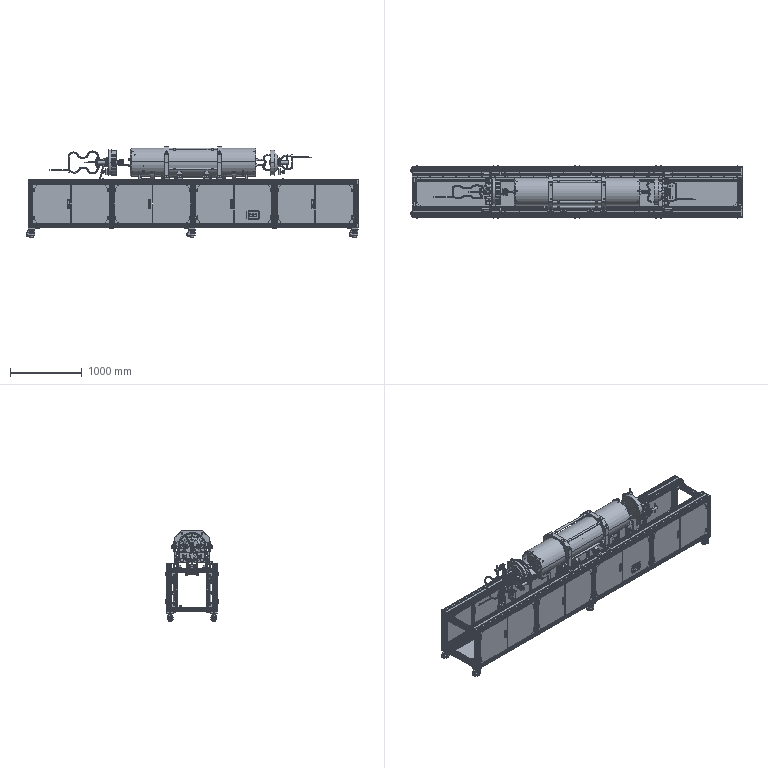Part | NX | features BREP 139 | 736 solids | 51179 faces | volume 268762420 mm3 | plane 24017 | cylinder 19731 | cone 2987 | torus 2045 | spline 1207 | sphere 1192 | commonest cylinder face diameters 0.1 x3584 18 x1464 17.4 x1440 6 x952 6.8 x882 2 x788